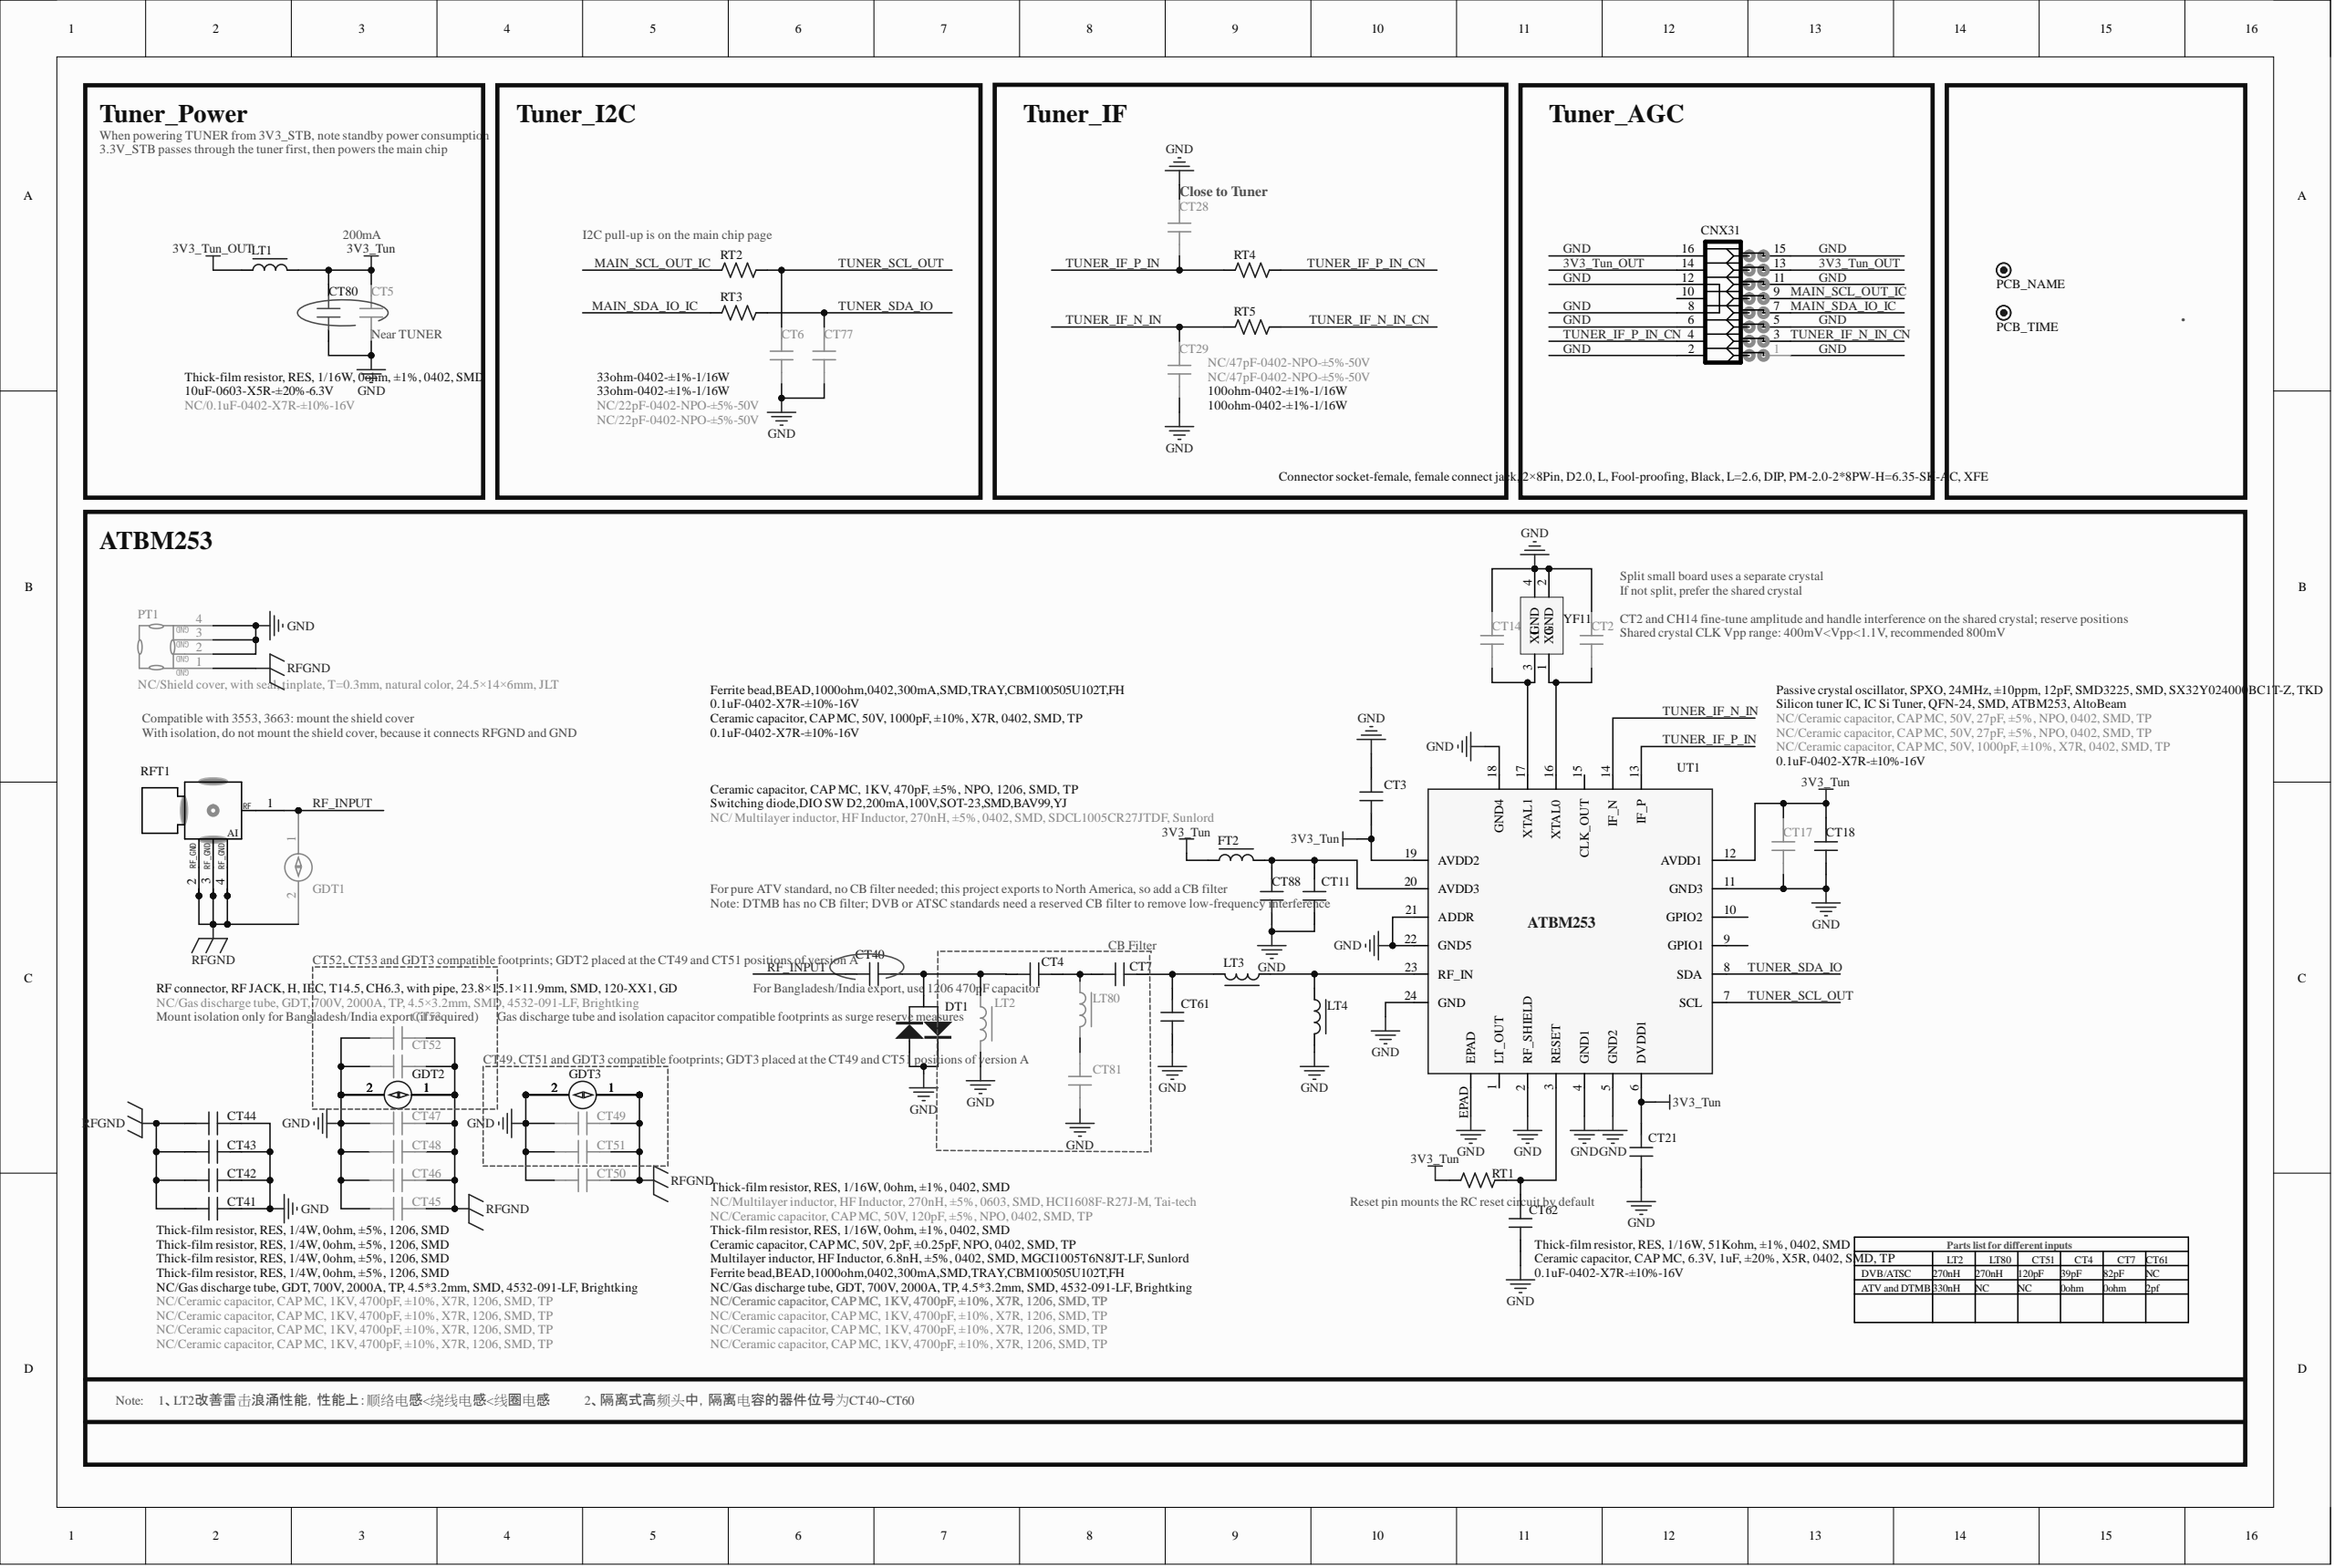Circuit board | Altium Designer | 541 parts | 263 nets | one sheet of the schematic
Parts on this sheet (reference | value | footprint):
CNX31 | Connector socket-female, female connect jack, 2×8Pin, D2.0, L, Fool-proofing, Black, L=2.6, DIP, PM-2.0-2*8PW-H=6.35-SK-AC, XFE | SIP2*8H/2.0DF-1
CT2 | NC/Ceramic capacitor, CAP MC, 50V, 27pF, ±5%, NPO, 0402, SMD, TP | C0402
CT3 | 0.1uF-0402-X7R-±10%-16V | C0402
CT4 | Thick-film resistor, RES, 1/16W, 0ohm, ±1%, 0402, SMD | C0402
CT5 | NC/0.1uF-0402-X7R-±10%-16V | C0402
CT6 | NC/22pF-0402-NPO-±5%-50V | C0402
CT7 | Thick-film resistor, RES, 1/16W, 0ohm, ±1%, 0402, SMD | C0402
CT11 | Ceramic capacitor, CAP MC, 50V, 1000pF, ±10%, X7R, 0402, SMD, TP | C0402
CT14 | NC/Ceramic capacitor, CAP MC, 50V, 27pF, ±5%, NPO, 0402, SMD, TP | C0402
CT17 | NC/Ceramic capacitor, CAP MC, 50V, 1000pF, ±10%, X7R, 0402, SMD, TP | C0402
CT18 | 0.1uF-0402-X7R-±10%-16V | C0402
CT21 | 0.1uF-0402-X7R-±10%-16V | C0402
CT28 | NC/47pF-0402-NPO-±5%-50V | C0402
CT29 | NC/47pF-0402-NPO-±5%-50V | C0402
CT40 | Ceramic capacitor, CAP MC, 1KV, 470pF, ±5%, NPO, 1206, SMD, TP | C1206
CT41 | Thick-film resistor, RES, 1/4W, 0ohm, ±5%, 1206, SMD | C1206
CT42 | Thick-film resistor, RES, 1/4W, 0ohm, ±5%, 1206, SMD | C1206
CT43 | Thick-film resistor, RES, 1/4W, 0ohm, ±5%, 1206, SMD | C1206
CT44 | Thick-film resistor, RES, 1/4W, 0ohm, ±5%, 1206, SMD | C1206
CT45 | NC/Ceramic capacitor, CAP MC, 1KV, 4700pF, ±10%, X7R, 1206, SMD, TP | C1206
CT46 | NC/Ceramic capacitor, CAP MC, 1KV, 4700pF, ±10%, X7R, 1206, SMD, TP | C1206
CT47 | NC/Ceramic capacitor, CAP MC, 1KV, 4700pF, ±10%, X7R, 1206, SMD, TP | C1206
CT48 | NC/Ceramic capacitor, CAP MC, 1KV, 4700pF, ±10%, X7R, 1206, SMD, TP | C1206
CT49 | NC/Ceramic capacitor, CAP MC, 1KV, 4700pF, ±10%, X7R, 1206, SMD, TP | C1206
CT50 | NC/Ceramic capacitor, CAP MC, 1KV, 4700pF, ±10%, X7R, 1206, SMD, TP | C1206
CT51 | NC/Ceramic capacitor, CAP MC, 1KV, 4700pF, ±10%, X7R, 1206, SMD, TP | C1206
CT52 | NC/Ceramic capacitor, CAP MC, 1KV, 4700pF, ±10%, X7R, 1206, SMD, TP | C1206
CT53 | NC/Ceramic capacitor, CAP MC, 1KV, 4700pF, ±10%, X7R, 1206, SMD, TP | C1206
CT61 | Ceramic capacitor, CAP MC, 50V, 2pF, ±0.25pF, NPO, 0402, SMD, TP | C0402
CT62 | Ceramic capacitor, CAP MC, 6.3V, 1uF, ±20%, X5R, 0402, SMD, TP | C0402
CT77 | NC/22pF-0402-NPO-±5%-50V | C0402
CT80 | 10uF-0603-X5R-±20%-6.3V | C0603
CT81 | NC/Ceramic capacitor, CAP MC, 50V, 120pF, ±5%, NPO, 0402, SMD, TP | C0402
CT88 | 0.1uF-0402-X7R-±10%-16V | C0402
DT1 | Switching diode,DIO SW D2,200mA,100V,SOT-23,SMD,BAV99,YJ | SO-23
FT2 | Ferrite bead,BEAD,1000ohm,0402,300mA,SMD,TRAY,CBM100505U102T,FH | L0402
GDT1 | NC/Gas discharge tube, GDT, 700V, 2000A, TP, 4.5×3.2mm, SMD, 4532-091-LF, Brightking | SMD4532-1
GDT2 | NC/Gas discharge tube, GDT, 700V, 2000A, TP, 4.5*3.2mm, SMD, 4532-091-LF, Brightking | SMD4532-1-C1206
GDT3 | NC/Gas discharge tube, GDT, 700V, 2000A, TP, 4.5*3.2mm, SMD, 4532-091-LF, Brightking | SMD4532-1-C1206
LT1 | Thick-film resistor, RES, 1/16W, 0ohm, ±1%, 0402, SMD | L0402
LT2 | NC/ Multilayer inductor, HF Inductor, 270nH, ±5%, 0402, SMD, SDCL1005CR27JTDF, Sunlord | L0402
LT3 | Multilayer inductor, HF Inductor, 6.8nH, ±5%, 0402, SMD, MGCI1005T6N8JT-LF, Sunlord | L0402
LT4 | Ferrite bead,BEAD,1000ohm,0402,300mA,SMD,TRAY,CBM100505U102T,FH | L0402
LT80 | NC/Multilayer inductor, HF Inductor, 270nH, ±5%, 0603, SMD, HCI1608F-R27J-M, Tai-tech | L0603
PT1 | NC/Shield cover, with seal, tinplate, T=0.3mm, natural color, 24.5×14×6mm, JLT | SHIELD(24.5*14*6)-TEMP-NG
RFT1 | RF connector, RF JACK, H, IEC, T14.5, CH6.3, with pipe, 23.8×15.1×11.9mm, SMD, 120-XX1, GD | T-12.8×10×9.3-IEC14.5-6.3
RT1 | Thick-film resistor, RES, 1/16W, 51Kohm, ±1%, 0402, SMD | R0402
RT2 | 33ohm-0402-±1%-1/16W | R0402
RT3 | 33ohm-0402-±1%-1/16W | R0402
RT4 | 100ohm-0402-±1%-1/16W | R0402
RT5 | 100ohm-0402-±1%-1/16W | R0402
UT1 | Silicon tuner IC, IC Si Tuner, QFN-24, SMD, ATBM253, AltoBeam | QFN24/0.4-1
YF11 | Passive crystal oscillator, SPXO, 24MHz, ±10ppm, 12pF, SMD3225, SMD, SX32Y024000BC1T-Z, TKD | XTAL-S-3
Nets of these parts (net: part-pin ...):
TUNER_SDA_IO: CT77-2 RT3-2 UT1-8
TUNER_SCL_OUT: CT6-2 RT2-2 UT1-7
TUNER_IF_P_IN_CN: CNX31-4 RT4-2
TUNER_IF_P_IN: CT28-2 RT4-1 UT1-13
TUNER_IF_N_IN_CN: CNX31-3 RT5-2
TUNER_IF_N_IN: CT29-1 RT5-1 UT1-14
RFGND: CT41-2 CT42-2 CT43-2 CT44-2 CT45-1 CT46-1 CT47-1 CT48-1 CT49-1 CT50-1 CT51-1 CT52-1 CT53-1 GDT1-2 GDT2-1 GDT3-1 PT1-1 RFT1-2 RFT1-3 RFT1-4
RF_INPUT: CT40-1 GDT1-1 RFT1-1
NetLT3_2: LT3-2 LT4-2 UT1-23
NetCT81_1: CT81-1 LT80-2
NetCT62_1: CT62-1 RT1-2 UT1-3
NetCT14_2: CT14-2 YF11-3 UT1-17
NetCT11_2: CT11-2 CT88-1 FT2-1 UT1-20
NetCT7_1: CT7-1 CT61-1 LT3-1
NetCT4_2: CT4-2 CT40-2 DT1-2 LT2-2
NetCT4_1: CT4-1 CT7-2 LT80-1
NetCT2_2: CT2-2 YF11-1 UT1-16
MAIN_SDA_IO_IC: CNX31-7 RT3-1
MAIN_SCL_OUT_IC: CNX31-9 RT2-1
GND: CNX31-1 CNX31-2 CNX31-5 CNX31-6 CNX31-8 CNX31-11 CNX31-12 CNX31-15 CNX31-16 CT2-1 CT3-1 CT5-2 CT6-1 CT11-1 CT14-1 CT17-2 CT18-1 CT21-1 CT28-1 CT29-2 CT41-1 CT42-1 CT43-1 CT44-1 CT45-2 CT46-2 CT47-2 CT48-2 CT49-2 CT50-2 CT51-2 CT52-2 CT53-2 CT61-2 CT62-2 CT77-1 CT80-1 CT81-2 CT88-2 DT1-1 DT1-3 GDT2-2 GDT3-2 LT2-1 LT4-1 PT1-2 PT1-3 PT1-4 YF11-2 YF11-4 UT1-2 UT1-4 UT1-5 UT1-11 UT1-18 UT1-21 UT1-22 UT1-24 UT1-EPAD
3V3_Tun_OUT: CNX31-13 CNX31-14 LT1-1
3V3_Tun: CT3-2 CT5-1 CT17-1 CT18-2 CT21-2 CT80-2 FT2-2 LT1-2 RT1-1 UT1-6 UT1-12 UT1-19